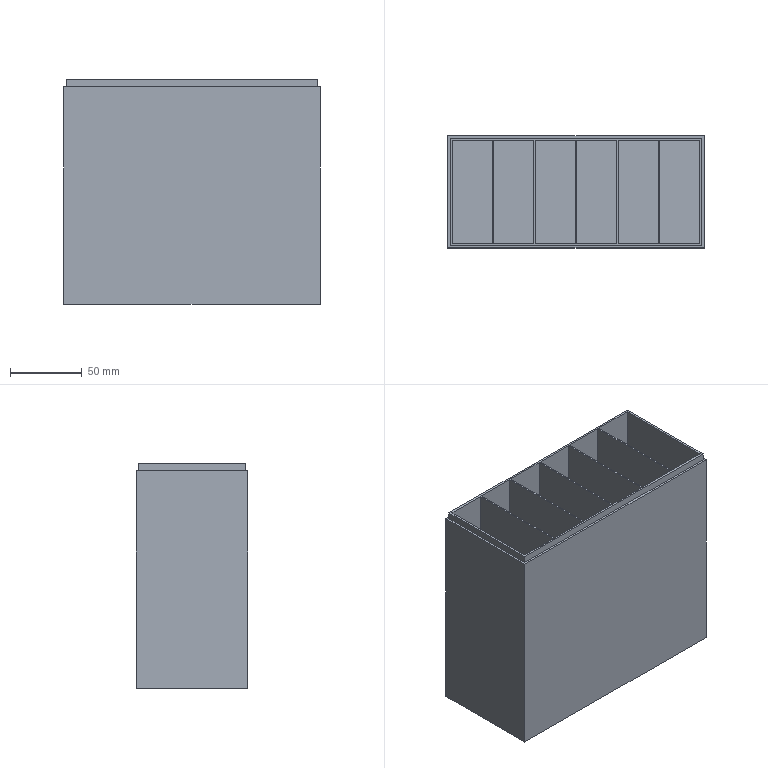Part | STEP file | 20AH housing | 1 solid | 41 faces | box 179 x 78 x 157 mm | volume 325440 mm3 | plane 41